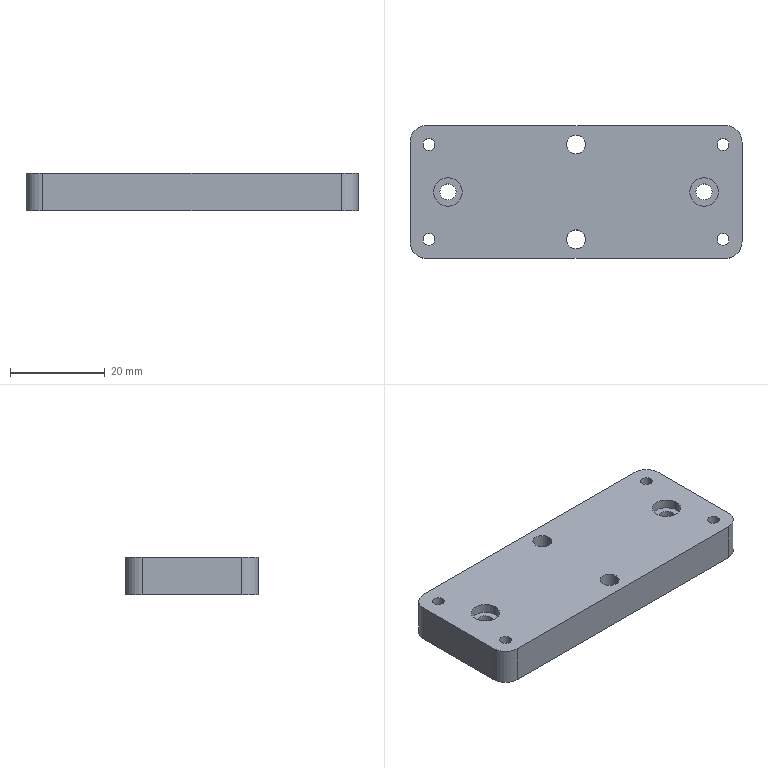Part | STEP file | 11-FG-SB01211 | 1 solid | 38 faces | box 70 x 28 x 8 mm | volume 14852 mm3 | cylinder 28 | plane 10 | commonest cylinder face diameters 2.5 x8 3.4 x4 4 x4 6 x4 6.5 x4 7 x4
STEP:
#1=CARTESIAN_POINT('',(-2.,-10.,8.));
#2=VERTEX_POINT('',#1);
#3=CARTESIAN_POINT('',(2.,-10.,8.));
#4=VERTEX_POINT('',#3);
#5=CARTESIAN_POINT('',(0.,-10.,8.));
#6=DIRECTION('',(0.,0.,1.));
#7=DIRECTION('',(1.,0.,0.));
#8=AXIS2_PLACEMENT_3D('',#5,#6,#7);
#9=CIRCLE('',#8,2.);
#10=EDGE_CURVE('',#2,#4,#9,.T.);
#11=ORIENTED_EDGE('',*,*,#10,.T.);
#12=CARTESIAN_POINT('',(2.,-10.,0.));
#13=VERTEX_POINT('',#12);
#14=CARTESIAN_POINT('',(2.,-10.,0.));
#15=DIRECTION('',(0.,0.,-1.));
#16=VECTOR('',#15,1000.);
#17=LINE('',#14,#16);
#18=EDGE_CURVE('',#4,#13,#17,.T.);
#19=ORIENTED_EDGE('',*,*,#18,.T.);
#20=CARTESIAN_POINT('',(-2.,-10.,0.));
#21=VERTEX_POINT('',#20);
#22=CARTESIAN_POINT('',(0.,-10.,0.));
#23=DIRECTION('',(0.,0.,-1.));
#24=DIRECTION('',(-1.,0.,0.));
#25=AXIS2_PLACEMENT_3D('',#22,#23,#24);
#26=CIRCLE('',#25,2.);
#27=EDGE_CURVE('',#13,#21,#26,.T.);
#28=ORIENTED_EDGE('',*,*,#27,.T.);
#29=CARTESIAN_POINT('',(-2.,-10.,0.));
#30=DIRECTION('',(0.,0.,-1.));
#31=VECTOR('',#30,1000.);
#32=LINE('',#29,#31);
#33=EDGE_CURVE('',#2,#21,#32,.T.);
#34=ORIENTED_EDGE('',*,*,#33,.F.);
#35=EDGE_LOOP('',(#11,#19,#28,#34));
#36=FACE_OUTER_BOUND('',#35,.T.);
#37=CARTESIAN_POINT('',(0.,-10.,0.));
#38=DIRECTION('',(0.,0.,-1.));
#39=DIRECTION('',(-1.,0.,0.));
#40=AXIS2_PLACEMENT_3D('',#37,#38,#39);
#41=CYLINDRICAL_SURFACE('',#40,2.);
#42=ADVANCED_FACE('',(#36),#41,.F.);
#43=CARTESIAN_POINT('',(-2.,10.,8.));
#44=VERTEX_POINT('',#43);
#45=CARTESIAN_POINT('',(2.,10.,8.));
#46=VERTEX_POINT('',#45);
#47=CARTESIAN_POINT('',(0.,10.,8.));
#48=DIRECTION('',(0.,0.,1.));
#49=DIRECTION('',(1.,0.,0.));
#50=AXIS2_PLACEMENT_3D('',#47,#48,#49);
#51=CIRCLE('',#50,2.);
#52=EDGE_CURVE('',#44,#46,#51,.T.);
#53=ORIENTED_EDGE('',*,*,#52,.T.);
#54=CARTESIAN_POINT('',(2.,10.,0.));
#55=VERTEX_POINT('',#54);
#56=CARTESIAN_POINT('',(2.,10.,0.));
#57=DIRECTION('',(0.,0.,-1.));
#58=VECTOR('',#57,1000.);
#59=LINE('',#56,#58);
#60=EDGE_CURVE('',#46,#55,#59,.T.);
#61=ORIENTED_EDGE('',*,*,#60,.T.);
#62=CARTESIAN_POINT('',(-2.,10.,0.));
#63=VERTEX_POINT('',#62);
#64=CARTESIAN_POINT('',(0.,10.,0.));
#65=DIRECTION('',(0.,0.,-1.));
#66=DIRECTION('',(-1.,0.,0.));
#67=AXIS2_PLACEMENT_3D('',#64,#65,#66);
#68=CIRCLE('',#67,2.);
#69=EDGE_CURVE('',#55,#63,#68,.T.);
#70=ORIENTED_EDGE('',*,*,#69,.T.);
#71=CARTESIAN_POINT('',(-2.,10.,0.));
#72=DIRECTION('',(0.,0.,-1.));
#73=VECTOR('',#72,1000.);
#74=LINE('',#71,#73);
#75=EDGE_CURVE('',#44,#63,#74,.T.);
#76=ORIENTED_EDGE('',*,*,#75,.F.);
#77=EDGE_LOOP('',(#53,#61,#70,#76));
#78=FACE_OUTER_BOUND('',#77,.T.);
#79=CARTESIAN_POINT('',(0.,10.,0.));
#80=DIRECTION('',(0.,0.,-1.));
#81=DIRECTION('',(-1.,0.,0.));
#82=AXIS2_PLACEMENT_3D('',#79,#80,#81);
#83=CYLINDRICAL_SURFACE('',#82,2.);
#84=ADVANCED_FACE('',(#78),#83,.F.);
#85=CARTESIAN_POINT('',(32.25,10.,8.));
#86=VERTEX_POINT('',#85);
#87=CARTESIAN_POINT('',(29.75,10.,8.));
#88=VERTEX_POINT('',#87);
#89=CARTESIAN_POINT('',(31.,10.,8.));
#90=DIRECTION('',(0.,0.,-1.));
#91=DIRECTION('',(-1.,0.,0.));
#92=AXIS2_PLACEMENT_3D('',#89,#90,#91);
#93=CIRCLE('',#92,1.25);
#94=EDGE_CURVE('',#86,#88,#93,.T.);
#95=ORIENTED_EDGE('',*,*,#94,.F.);
#96=CARTESIAN_POINT('',(32.25,10.,0.));
#97=VERTEX_POINT('',#96);
#98=CARTESIAN_POINT('',(32.25,10.,0.));
#99=DIRECTION('',(0.,0.,-1.));
#100=VECTOR('',#99,1000.);
#101=LINE('',#98,#100);
#102=EDGE_CURVE('',#86,#97,#101,.T.);
#103=ORIENTED_EDGE('',*,*,#102,.T.);
#104=CARTESIAN_POINT('',(29.75,10.,0.));
#105=VERTEX_POINT('',#104);
#106=CARTESIAN_POINT('',(31.,10.,0.));
#107=DIRECTION('',(0.,0.,-1.));
#108=DIRECTION('',(-1.,0.,0.));
#109=AXIS2_PLACEMENT_3D('',#106,#107,#108);
#110=CIRCLE('',#109,1.25);
#111=EDGE_CURVE('',#97,#105,#110,.T.);
#112=ORIENTED_EDGE('',*,*,#111,.T.);
#113=CARTESIAN_POINT('',(29.75,10.,0.));
#114=DIRECTION('',(0.,0.,-1.));
#115=VECTOR('',#114,1000.);
#116=LINE('',#113,#115);
#117=EDGE_CURVE('',#88,#105,#116,.T.);
#118=ORIENTED_EDGE('',*,*,#117,.F.);
#119=EDGE_LOOP('',(#95,#103,#112,#118));
#120=FACE_OUTER_BOUND('',#119,.T.);
#121=CARTESIAN_POINT('',(31.,10.,0.));
#122=DIRECTION('',(0.,0.,-1.));
#123=DIRECTION('',(-1.,0.,0.));
#124=AXIS2_PLACEMENT_3D('',#121,#122,#123);
#125=CYLINDRICAL_SURFACE('',#124,1.25);
#126=ADVANCED_FACE('',(#120),#125,.F.);
#127=CARTESIAN_POINT('',(32.25,-10.,8.));
#128=VERTEX_POINT('',#127);
#129=CARTESIAN_POINT('',(29.75,-10.,8.));
#130=VERTEX_POINT('',#129);
#131=CARTESIAN_POINT('',(31.,-10.,8.));
#132=DIRECTION('',(0.,0.,-1.));
#133=DIRECTION('',(-1.,0.,0.));
#134=AXIS2_PLACEMENT_3D('',#131,#132,#133);
#135=CIRCLE('',#134,1.25);
#136=EDGE_CURVE('',#128,#130,#135,.T.);
#137=ORIENTED_EDGE('',*,*,#136,.F.);
#138=CARTESIAN_POINT('',(32.25,-10.,0.));
#139=VERTEX_POINT('',#138);
#140=CARTESIAN_POINT('',(32.25,-10.,0.));
#141=DIRECTION('',(0.,0.,-1.));
#142=VECTOR('',#141,1000.);
#143=LINE('',#140,#142);
#144=EDGE_CURVE('',#128,#139,#143,.T.);
#145=ORIENTED_EDGE('',*,*,#144,.T.);
#146=CARTESIAN_POINT('',(29.75,-10.,0.));
#147=VERTEX_POINT('',#146);
#148=CARTESIAN_POINT('',(31.,-10.,0.));
#149=DIRECTION('',(0.,0.,-1.));
#150=DIRECTION('',(-1.,0.,0.));
#151=AXIS2_PLACEMENT_3D('',#148,#149,#150);
#152=CIRCLE('',#151,1.25);
#153=EDGE_CURVE('',#139,#147,#152,.T.);
#154=ORIENTED_EDGE('',*,*,#153,.T.);
#155=CARTESIAN_POINT('',(29.75,-10.,0.));
#156=DIRECTION('',(0.,0.,-1.));
#157=VECTOR('',#156,1000.);
#158=LINE('',#155,#157);
#159=EDGE_CURVE('',#130,#147,#158,.T.);
#160=ORIENTED_EDGE('',*,*,#159,.F.);
#161=EDGE_LOOP('',(#137,#145,#154,#160));
#162=FACE_OUTER_BOUND('',#161,.T.);
#163=CARTESIAN_POINT('',(31.,-10.,0.));
#164=DIRECTION('',(0.,0.,-1.));
#165=DIRECTION('',(-1.,0.,0.));
#166=AXIS2_PLACEMENT_3D('',#163,#164,#165);
#167=CYLINDRICAL_SURFACE('',#166,1.25);
#168=ADVANCED_FACE('',(#162),#167,.F.);
#169=CARTESIAN_POINT('',(-29.75,-10.,8.));
#170=VERTEX_POINT('',#169);
#171=CARTESIAN_POINT('',(-32.25,-10.,8.));
#172=VERTEX_POINT('',#171);
#173=CARTESIAN_POINT('',(-31.,-10.,8.));
#174=DIRECTION('',(0.,0.,-1.));
#175=DIRECTION('',(-1.,0.,0.));
#176=AXIS2_PLACEMENT_3D('',#173,#174,#175);
#177=CIRCLE('',#176,1.25);
#178=EDGE_CURVE('',#170,#172,#177,.T.);
#179=ORIENTED_EDGE('',*,*,#178,.F.);
#180=CARTESIAN_POINT('',(-29.75,-10.,0.));
#181=VERTEX_POINT('',#180);
#182=CARTESIAN_POINT('',(-29.75,-10.,0.));
#183=DIRECTION('',(0.,0.,-1.));
#184=VECTOR('',#183,1000.);
#185=LINE('',#182,#184);
#186=EDGE_CURVE('',#170,#181,#185,.T.);
#187=ORIENTED_EDGE('',*,*,#186,.T.);
#188=CARTESIAN_POINT('',(-32.25,-10.,0.));
#189=VERTEX_POINT('',#188);
#190=CARTESIAN_POINT('',(-31.,-10.,0.));
#191=DIRECTION('',(0.,0.,-1.));
#192=DIRECTION('',(-1.,0.,0.));
#193=AXIS2_PLACEMENT_3D('',#190,#191,#192);
#194=CIRCLE('',#193,1.25);
#195=EDGE_CURVE('',#181,#189,#194,.T.);
#196=ORIENTED_EDGE('',*,*,#195,.T.);
#197=CARTESIAN_POINT('',(-32.25,-10.,0.));
#198=DIRECTION('',(0.,0.,-1.));
#199=VECTOR('',#198,1000.);
#200=LINE('',#197,#199);
#201=EDGE_CURVE('',#172,#189,#200,.T.);
#202=ORIENTED_EDGE('',*,*,#201,.F.);
#203=EDGE_LOOP('',(#179,#187,#196,#202));
#204=FACE_OUTER_BOUND('',#203,.T.);
#205=CARTESIAN_POINT('',(-31.,-10.,0.));
#206=DIRECTION('',(0.,0.,-1.));
#207=DIRECTION('',(-1.,0.,0.));
#208=AXIS2_PLACEMENT_3D('',#205,#206,#207);
#209=CYLINDRICAL_SURFACE('',#208,1.25);
#210=ADVANCED_FACE('',(#204),#209,.F.);
#211=CARTESIAN_POINT('',(-29.75,10.,8.));
#212=VERTEX_POINT('',#211);
#213=CARTESIAN_POINT('',(-32.25,10.,8.));
#214=VERTEX_POINT('',#213);
#215=CARTESIAN_POINT('',(-31.,10.,8.));
#216=DIRECTION('',(0.,0.,-1.));
#217=DIRECTION('',(-1.,0.,0.));
#218=AXIS2_PLACEMENT_3D('',#215,#216,#217);
#219=CIRCLE('',#218,1.25);
#220=EDGE_CURVE('',#212,#214,#219,.T.);
#221=ORIENTED_EDGE('',*,*,#220,.F.);
#222=CARTESIAN_POINT('',(-29.75,10.,0.));
#223=VERTEX_POINT('',#222);
#224=CARTESIAN_POINT('',(-29.75,10.,0.));
#225=DIRECTION('',(0.,0.,-1.));
#226=VECTOR('',#225,1000.);
#227=LINE('',#224,#226);
#228=EDGE_CURVE('',#212,#223,#227,.T.);
#229=ORIENTED_EDGE('',*,*,#228,.T.);
#230=CARTESIAN_POINT('',(-32.25,10.,0.));
#231=VERTEX_POINT('',#230);
#232=CARTESIAN_POINT('',(-31.,10.,0.));
#233=DIRECTION('',(0.,0.,-1.));
#234=DIRECTION('',(-1.,0.,0.));
#235=AXIS2_PLACEMENT_3D('',#232,#233,#234);
#236=CIRCLE('',#235,1.25);
#237=EDGE_CURVE('',#223,#231,#236,.T.);
#238=ORIENTED_EDGE('',*,*,#237,.T.);
#239=CARTESIAN_POINT('',(-32.25,10.,0.));
#240=DIRECTION('',(0.,0.,-1.));
#241=VECTOR('',#240,1000.);
#242=LINE('',#239,#241);
#243=EDGE_CURVE('',#214,#231,#242,.T.);
#244=ORIENTED_EDGE('',*,*,#243,.F.);
#245=EDGE_LOOP('',(#221,#229,#238,#244));
#246=FACE_OUTER_BOUND('',#245,.T.);
#247=CARTESIAN_POINT('',(-31.,10.,0.));
#248=DIRECTION('',(0.,0.,-1.));
#249=DIRECTION('',(-1.,0.,0.));
#250=AXIS2_PLACEMENT_3D('',#247,#248,#249);
#251=CYLINDRICAL_SURFACE('',#250,1.25);
#252=ADVANCED_FACE('',(#246),#251,.F.);
#253=CARTESIAN_POINT('',(-23.75,0.,3.4));
#254=VERTEX_POINT('',#253);
#255=CARTESIAN_POINT('',(-30.25,0.,3.4));
#256=VERTEX_POINT('',#255);
#257=CARTESIAN_POINT('',(-27.,0.,3.4));
#258=DIRECTION('',(0.,0.,-1.));
#259=DIRECTION('',(-1.,0.,0.));
#260=AXIS2_PLACEMENT_3D('',#257,#258,#259);
#261=CIRCLE('',#260,3.25);
#262=EDGE_CURVE('',#254,#256,#261,.T.);
#263=ORIENTED_EDGE('',*,*,#262,.F.);
#264=CARTESIAN_POINT('',(-23.75,0.,0.));
#265=VERTEX_POINT('',#264);
#266=CARTESIAN_POINT('',(-23.75,0.,0.));
#267=DIRECTION('',(0.,0.,-1.));
#268=VECTOR('',#267,1000.);
#269=LINE('',#266,#268);
#270=EDGE_CURVE('',#254,#265,#269,.T.);
#271=ORIENTED_EDGE('',*,*,#270,.T.);
#272=CARTESIAN_POINT('',(-30.25,0.,0.));
#273=VERTEX_POINT('',#272);
#274=CARTESIAN_POINT('',(-27.,0.,0.));
#275=DIRECTION('',(0.,0.,-1.));
#276=DIRECTION('',(-1.,0.,0.));
#277=AXIS2_PLACEMENT_3D('',#274,#275,#276);
#278=CIRCLE('',#277,3.25);
#279=EDGE_CURVE('',#265,#273,#278,.T.);
#280=ORIENTED_EDGE('',*,*,#279,.T.);
#281=CARTESIAN_POINT('',(-30.25,0.,0.));
#282=DIRECTION('',(0.,0.,-1.));
#283=VECTOR('',#282,1000.);
#284=LINE('',#281,#283);
#285=EDGE_CURVE('',#256,#273,#284,.T.);
#286=ORIENTED_EDGE('',*,*,#285,.F.);
#287=EDGE_LOOP('',(#263,#271,#280,#286));
#288=FACE_OUTER_BOUND('',#287,.T.);
#289=CARTESIAN_POINT('',(-27.,0.,0.));
#290=DIRECTION('',(0.,0.,-1.));
#291=DIRECTION('',(-1.,0.,0.));
#292=AXIS2_PLACEMENT_3D('',#289,#290,#291);
#293=CYLINDRICAL_SURFACE('',#292,3.25);
#294=ADVANCED_FACE('',(#288),#293,.F.);
#295=CARTESIAN_POINT('',(-25.3,0.,6.));
#296=VERTEX_POINT('',#295);
#297=CARTESIAN_POINT('',(-28.7,0.,6.));
#298=VERTEX_POINT('',#297);
#299=CARTESIAN_POINT('',(-27.,0.,6.));
#300=DIRECTION('',(0.,0.,-1.));
#301=DIRECTION('',(-1.,0.,0.));
#302=AXIS2_PLACEMENT_3D('',#299,#300,#301);
#303=CIRCLE('',#302,1.7);
#304=EDGE_CURVE('',#296,#298,#303,.T.);
#305=ORIENTED_EDGE('',*,*,#304,.F.);
#306=CARTESIAN_POINT('',(-25.3,0.,3.4));
#307=VERTEX_POINT('',#306);
#308=CARTESIAN_POINT('',(-25.3,0.,0.));
#309=DIRECTION('',(0.,0.,-1.));
#310=VECTOR('',#309,1000.);
#311=LINE('',#308,#310);
#312=EDGE_CURVE('',#296,#307,#311,.T.);
#313=ORIENTED_EDGE('',*,*,#312,.T.);
#314=CARTESIAN_POINT('',(-28.7,0.,3.4));
#315=VERTEX_POINT('',#314);
#316=CARTESIAN_POINT('',(-27.,0.,3.4));
#317=DIRECTION('',(0.,0.,-1.));
#318=DIRECTION('',(-1.,0.,0.));
#319=AXIS2_PLACEMENT_3D('',#316,#317,#318);
#320=CIRCLE('',#319,1.7);
#321=EDGE_CURVE('',#307,#315,#320,.T.);
#322=ORIENTED_EDGE('',*,*,#321,.T.);
#323=CARTESIAN_POINT('',(-28.7,0.,0.));
#324=DIRECTION('',(0.,0.,-1.));
#325=VECTOR('',#324,1000.);
#326=LINE('',#323,#325);
#327=EDGE_CURVE('',#298,#315,#326,.T.);
#328=ORIENTED_EDGE('',*,*,#327,.F.);
#329=EDGE_LOOP('',(#305,#313,#322,#328));
#330=FACE_OUTER_BOUND('',#329,.T.);
#331=CARTESIAN_POINT('',(-27.,0.,0.));
#332=DIRECTION('',(0.,0.,-1.));
#333=DIRECTION('',(-1.,0.,0.));
#334=AXIS2_PLACEMENT_3D('',#331,#332,#333);
#335=CYLINDRICAL_SURFACE('',#334,1.7);
#336=ADVANCED_FACE('',(#330),#335,.F.);
#337=CARTESIAN_POINT('',(30.25,0.,3.4));
#338=VERTEX_POINT('',#337);
#339=CARTESIAN_POINT('',(23.75,0.,3.4));
#340=VERTEX_POINT('',#339);
#341=CARTESIAN_POINT('',(27.,0.,3.4));
#342=DIRECTION('',(0.,0.,-1.));
#343=DIRECTION('',(-1.,0.,0.));
#344=AXIS2_PLACEMENT_3D('',#341,#342,#343);
#345=CIRCLE('',#344,3.25);
#346=EDGE_CURVE('',#338,#340,#345,.T.);
#347=ORIENTED_EDGE('',*,*,#346,.F.);
#348=CARTESIAN_POINT('',(30.25,0.,0.));
#349=VERTEX_POINT('',#348);
#350=CARTESIAN_POINT('',(30.25,0.,0.));
#351=DIRECTION('',(0.,0.,-1.));
#352=VECTOR('',#351,1000.);
#353=LINE('',#350,#352);
#354=EDGE_CURVE('',#338,#349,#353,.T.);
#355=ORIENTED_EDGE('',*,*,#354,.T.);
#356=CARTESIAN_POINT('',(23.75,0.,0.));
#357=VERTEX_POINT('',#356);
#358=CARTESIAN_POINT('',(27.,0.,0.));
#359=DIRECTION('',(0.,0.,-1.));
#360=DIRECTION('',(-1.,0.,0.));
#361=AXIS2_PLACEMENT_3D('',#358,#359,#360);
#362=CIRCLE('',#361,3.25);
#363=EDGE_CURVE('',#349,#357,#362,.T.);
#364=ORIENTED_EDGE('',*,*,#363,.T.);
#365=CARTESIAN_POINT('',(23.75,0.,0.));
#366=DIRECTION('',(0.,0.,-1.));
#367=VECTOR('',#366,1000.);
#368=LINE('',#365,#367);
#369=EDGE_CURVE('',#340,#357,#368,.T.);
#370=ORIENTED_EDGE('',*,*,#369,.F.);
#371=EDGE_LOOP('',(#347,#355,#364,#370));
#372=FACE_OUTER_BOUND('',#371,.T.);
#373=CARTESIAN_POINT('',(27.,0.,0.));
#374=DIRECTION('',(0.,0.,-1.));
#375=DIRECTION('',(-1.,0.,0.));
#376=AXIS2_PLACEMENT_3D('',#373,#374,#375);
#377=CYLINDRICAL_SURFACE('',#376,3.25);
#378=ADVANCED_FACE('',(#372),#377,.F.);
#379=CARTESIAN_POINT('',(25.3,0.,6.));
#380=VERTEX_POINT('',#379);
#381=CARTESIAN_POINT('',(28.7,0.,6.));
#382=VERTEX_POINT('',#381);
#383=CARTESIAN_POINT('',(27.,0.,6.));
#384=DIRECTION('',(0.,0.,1.));
#385=DIRECTION('',(1.,0.,0.));
#386=AXIS2_PLACEMENT_3D('',#383,#384,#385);
#387=CIRCLE('',#386,1.7);
#388=EDGE_CURVE('',#380,#382,#387,.T.);
#389=ORIENTED_EDGE('',*,*,#388,.T.);
#390=CARTESIAN_POINT('',(28.7,0.,3.4));
#391=VERTEX_POINT('',#390);
#392=CARTESIAN_POINT('',(28.7,0.,0.));
#393=DIRECTION('',(0.,0.,-1.));
#394=VECTOR('',#393,1000.);
#395=LINE('',#392,#394);
#396=EDGE_CURVE('',#382,#391,#395,.T.);
#397=ORIENTED_EDGE('',*,*,#396,.T.);
#398=CARTESIAN_POINT('',(25.3,0.,3.4));
#399=VERTEX_POINT('',#398);
#400=CARTESIAN_POINT('',(27.,0.,3.4));
#401=DIRECTION('',(0.,0.,-1.));
#402=DIRECTION('',(-1.,0.,0.));
#403=AXIS2_PLACEMENT_3D('',#400,#401,#402);
#404=CIRCLE('',#403,1.7);
#405=EDGE_CURVE('',#391,#399,#404,.T.);
#406=ORIENTED_EDGE('',*,*,#405,.T.);
#407=CARTESIAN_POINT('',(25.3,0.,0.));
#408=DIRECTION('',(0.,0.,-1.));
#409=VECTOR('',#408,1000.);
#410=LINE('',#407,#409);
#411=EDGE_CURVE('',#380,#399,#410,.T.);
#412=ORIENTED_EDGE('',*,*,#411,.F.);
#413=EDGE_LOOP('',(#389,#397,#406,#412));
#414=FACE_OUTER_BOUND('',#413,.T.);
#415=CARTESIAN_POINT('',(27.,0.,0.));
#416=DIRECTION('',(0.,0.,-1.));
#417=DIRECTION('',(-1.,0.,0.));
#418=AXIS2_PLACEMENT_3D('',#415,#416,#417);
#419=CYLINDRICAL_SURFACE('',#418,1.7);
#420=ADVANCED_FACE('',(#414),#419,.F.);
#421=CARTESIAN_POINT('',(-30.,0.,6.));
#422=VERTEX_POINT('',#421);
#423=CARTESIAN_POINT('',(-24.,0.,6.));
#424=VERTEX_POINT('',#423);
#425=CARTESIAN_POINT('',(-27.,0.,6.));
#426=DIRECTION('',(0.,0.,1.));
#427=DIRECTION('',(-1.,0.,0.));
#428=AXIS2_PLACEMENT_3D('',#425,#426,#427);
#429=CIRCLE('',#428,3.);
#430=EDGE_CURVE('',#422,#424,#429,.T.);
#431=ORIENTED_EDGE('',*,*,#430,.F.);
#432=CARTESIAN_POINT('',(-30.,0.,8.));
#433=VERTEX_POINT('',#432);
#434=CARTESIAN_POINT('',(-30.,0.,6.));
#435=DIRECTION('',(0.,0.,1.));
#436=VECTOR('',#435,1000.);
#437=LINE('',#434,#436);
#438=EDGE_CURVE('',#422,#433,#437,.T.);
#439=ORIENTED_EDGE('',*,*,#438,.T.);
#440=CARTESIAN_POINT('',(-24.,0.,8.));
#441=VERTEX_POINT('',#440);
#442=CARTESIAN_POINT('',(-27.,0.,8.));
#443=DIRECTION('',(0.,0.,1.));
#444=DIRECTION('',(-1.,0.,0.));
#445=AXIS2_PLACEMENT_3D('',#442,#443,#444);
#446=CIRCLE('',#445,3.);
#447=EDGE_CURVE('',#433,#441,#446,.T.);
#448=ORIENTED_EDGE('',*,*,#447,.T.);
#449=CARTESIAN_POINT('',(-24.,0.,6.));
#450=DIRECTION('',(0.,0.,1.));
#451=VECTOR('',#450,1000.);
#452=LINE('',#449,#451);
#453=EDGE_CURVE('',#424,#441,#452,.T.);
#454=ORIENTED_EDGE('',*,*,#453,.F.);
#455=EDGE_LOOP('',(#431,#439,#448,#454));
#456=FACE_OUTER_BOUND('',#455,.T.);
#457=CARTESIAN_POINT('',(-27.,0.,6.));
#458=DIRECTION('',(0.,0.,1.));
#459=DIRECTION('',(1.,0.,0.));
#460=AXIS2_PLACEMENT_3D('',#457,#458,#459);
#461=CYLINDRICAL_SURFACE('',#460,3.);
#462=ADVANCED_FACE('',(#456),#461,.F.);
#463=CARTESIAN_POINT('',(24.,0.,6.));
#464=VERTEX_POINT('',#463);
#465=CARTESIAN_POINT('',(30.,0.,6.));
#466=VERTEX_POINT('',#465);
#467=CARTESIAN_POINT('',(27.,0.,6.));
#468=DIRECTION('',(0.,0.,1.));
#469=DIRECTION('',(1.,0.,0.));
#470=AXIS2_PLACEMENT_3D('',#467,#468,#469);
#471=CIRCLE('',#470,3.);
#472=EDGE_CURVE('',#464,#466,#471,.T.);
#473=ORIENTED_EDGE('',*,*,#472,.F.);
#474=CARTESIAN_POINT('',(24.,0.,8.));
#475=VERTEX_POINT('',#474);
#476=CARTESIAN_POINT('',(24.,0.,6.));
#477=DIRECTION('',(0.,0.,1.));
#478=VECTOR('',#477,1000.);
#479=LINE('',#476,#478);
#480=EDGE_CURVE('',#464,#475,#479,.T.);
#481=ORIENTED_EDGE('',*,*,#480,.T.);
#482=CARTESIAN_POINT('',(30.,0.,8.));
#483=VERTEX_POINT('',#482);
#484=CARTESIAN_POINT('',(27.,0.,8.));
#485=DIRECTION('',(0.,0.,1.));
#486=DIRECTION('',(1.,0.,0.));
#487=AXIS2_PLACEMENT_3D('',#484,#485,#486);
#488=CIRCLE('',#487,3.);
#489=EDGE_CURVE('',#475,#483,#488,.T.);
#490=ORIENTED_EDGE('',*,*,#489,.T.);
#491=CARTESIAN_POINT('',(30.,0.,6.));
#492=DIRECTION('',(0.,0.,1.));
#493=VECTOR('',#492,1000.);
#494=LINE('',#491,#493);
#495=EDGE_CURVE('',#466,#483,#494,.T.);
#496=ORIENTED_EDGE('',*,*,#495,.F.);
#497=EDGE_LOOP('',(#473,#481,#490,#496));
#498=FACE_OUTER_BOUND('',#497,.T.);
#499=CARTESIAN_POINT('',(27.,0.,6.));
#500=DIRECTION('',(0.,0.,1.));
#501=DIRECTION('',(1.,0.,0.));
#502=AXIS2_PLACEMENT_3D('',#499,#500,#501);
#503=CYLINDRICAL_SURFACE('',#502,3.);
#504=ADVANCED_FACE('',(#498),#503,.F.);
#505=CARTESIAN_POINT('',(35.,-10.5,0.));
#506=VERTEX_POINT('',#505);
#507=CARTESIAN_POINT('',(35.,10.5,0.));
#508=VERTEX_POINT('',#507);
#509=CARTESIAN_POINT('',(35.,14.,0.));
#510=DIRECTION('',(0.,1.,0.));
#511=VECTOR('',#510,1000.);
#512=LINE('',#509,#511);
#513=EDGE_CURVE('',#506,#508,#512,.T.);
#514=ORIENTED_EDGE('',*,*,#513,.T.);
#515=CARTESIAN_POINT('',(35.,10.5,8.));
#516=VERTEX_POINT('',#515);
#517=CARTESIAN_POINT('',(35.,10.5,8.));
#518=DIRECTION('',(0.,0.,1.));
#519=VECTOR('',#518,1000.);
#520=LINE('',#517,#519);
#521=EDGE_CURVE('',#508,#516,#520,.T.);
#522=ORIENTED_EDGE('',*,*,#521,.T.);
#523=CARTESIAN_POINT('',(35.,-10.5,8.));
#524=VERTEX_POINT('',#523);
#525=CARTESIAN_POINT('',(35.,14.,8.));
#526=DIRECTION('',(0.,1.,0.));
#527=VECTOR('',#526,1000.);
#528=LINE('',#525,#527);
#529=EDGE_CURVE('',#524,#516,#528,.T.);
#530=ORIENTED_EDGE('',*,*,#529,.F.);
#531=CARTESIAN_POINT('',(35.,-10.5,8.));
#532=DIRECTION('',(0.,0.,-1.));
#533=VECTOR('',#532,1000.);
#534=LINE('',#531,#533);
#535=EDGE_CURVE('',#524,#506,#534,.T.);
#536=ORIENTED_EDGE('',*,*,#535,.T.);
#537=EDGE_LOOP('',(#514,#522,#530,#536));
#538=FACE_OUTER_BOUND('',#537,.T.);
#539=CARTESIAN_POINT('',(35.,14.,8.));
#540=DIRECTION('',(-1.,0.,0.));
#541=DIRECTION('',(0.,0.,1.));
#542=AXIS2_PLACEMENT_3D('',#539,#540,#541);
#543=PLANE('',#542);
#544=ADVANCED_FACE('',(#538),#543,.F.);
#545=CARTESIAN_POINT('',(31.5,14.,8.));
#546=VERTEX_POINT('',#545);
#547=CARTESIAN_POINT('',(-31.5,14.,8.));
#548=VERTEX_POINT('',#547);
#549=CARTESIAN_POINT('',(-35.,14.,8.));
#550=DIRECTION('',(-1.,0.,0.));
#551=VECTOR('',#550,1000.);
#552=LINE('',#549,#551);
#553=EDGE_CURVE('',#546,#548,#552,.T.);
#554=ORIENTED_EDGE('',*,*,#553,.F.);
#555=CARTESIAN_POINT('',(31.5,14.,0.));
#556=VERTEX_POINT('',#555);
#557=CARTESIAN_POINT('',(31.5,14.,8.));
#558=DIRECTION('',(0.,0.,-1.));
#559=VECTOR('',#558,1000.);
#560=LINE('',#557,#559);
#561=EDGE_CURVE('',#546,#556,#560,.T.);
#562=ORIENTED_EDGE('',*,*,#561,.T.);
#563=CARTESIAN_POINT('',(-31.5,14.,0.));
#564=VERTEX_POINT('',#563);
#565=CARTESIAN_POINT('',(-35.,14.,0.));
#566=DIRECTION('',(-1.,0.,0.));
#567=VECTOR('',#566,1000.);
#568=LINE('',#565,#567);
#569=EDGE_CURVE('',#556,#564,#568,.T.);
#570=ORIENTED_EDGE('',*,*,#569,.T.);
#571=CARTESIAN_POINT('',(-31.5,14.,8.));
#572=DIRECTION('',(0.,0.,1.));
#573=VECTOR('',#572,1000.);
#574=LINE('',#571,#573);
#575=EDGE_CURVE('',#564,#548,#574,.T.);
#576=ORIENTED_EDGE('',*,*,#575,.T.);
#577=EDGE_LOOP('',(#554,#562,#570,#576));
#578=FACE_OUTER_BOUND('',#577,.T.);
#579=CARTESIAN_POINT('',(-35.,14.,8.));
#580=DIRECTION('',(0.,-1.,0.));
#581=DIRECTION('',(0.,0.,-1.));
#582=AXIS2_PLACEMENT_3D('',#579,#580,#581);
#583=PLANE('',#582);
#584=ADVANCED_FACE('',(#578),#583,.F.);
#585=CARTESIAN_POINT('',(-35.,10.5,0.));
#586=VERTEX_POINT('',#585);
#587=CARTESIAN_POINT('',(-35.,-10.5,0.));
#588=VERTEX_POINT('',#587);
#589=CARTESIAN_POINT('',(-35.,14.,0.));
#590=DIRECTION('',(0.,-1.,0.));
#591=VECTOR('',#590,1000.);
#592=LINE('',#589,#591);
#593=EDGE_CURVE('',#586,#588,#592,.T.);
#594=ORIENTED_EDGE('',*,*,#593,.T.);
#595=CARTESIAN_POINT('',(-35.,-10.5,8.));
#596=VERTEX_POINT('',#595);
#597=CARTESIAN_POINT('',(-35.,-10.5,8.));
#598=DIRECTION('',(0.,0.,1.));
#599=VECTOR('',#598,1000.);
#600=LINE('',#597,#599);
#601=EDGE_CURVE('',#588,#596,#600,.T.);
#602=ORIENTED_EDGE('',*,*,#601,.T.);
#603=CARTESIAN_POINT('',(-35.,10.5,8.));
#604=VERTEX_POINT('',#603);
#605=CARTESIAN_POINT('',(-35.,14.,8.));
#606=DIRECTION('',(0.,-1.,0.));
#607=VECTOR('',#606,1000.);
#608=LINE('',#605,#607);
#609=EDGE_CURVE('',#604,#596,#608,.T.);
#610=ORIENTED_EDGE('',*,*,#609,.F.);
#611=CARTESIAN_POINT('',(-35.,10.5,8.));
#612=DIRECTION('',(0.,0.,-1.));
#613=VECTOR('',#612,1000.);
#614=LINE('',#611,#613);
#615=EDGE_CURVE('',#604,#586,#614,.T.);
#616=ORIENTED_EDGE('',*,*,#615,.T.);
#617=EDGE_LOOP('',(#594,#602,#610,#616));
#618=FACE_OUTER_BOUND('',#617,.T.);
#619=CARTESIAN_POINT('',(-35.,14.,8.));
#620=DIRECTION('',(1.,0.,0.));
#621=DIRECTION('',(0.,1.,0.));
#622=AXIS2_PLACEMENT_3D('',#619,#620,#621);
#623=PLANE('',#622);
#624=ADVANCED_FACE('',(#618),#623,.F.);
#625=CARTESIAN_POINT('',(-31.5,-14.,0.));
#626=VERTEX_POINT('',#625);
#627=CARTESIAN_POINT('',(31.5,-14.,0.));
#628=VERTEX_POINT('',#627);
#629=CARTESIAN_POINT('',(-35.,-14.,0.));
#630=DIRECTION('',(1.,0.,0.));
#631=VECTOR('',#630,1000.);
#632=LINE('',#629,#631);
#633=EDGE_CURVE('',#626,#628,#632,.T.);
#634=ORIENTED_EDGE('',*,*,#633,.T.);
#635=CARTESIAN_POINT('',(31.5,-14.,8.));
#636=VERTEX_POINT('',#635);
#637=CARTESIAN_POINT('',(31.5,-14.,8.));
#638=DIRECTION('',(0.,0.,1.));
#639=VECTOR('',#638,1000.);
#640=LINE('',#637,#639);
#641=EDGE_CURVE('',#628,#636,#640,.T.);
#642=ORIENTED_EDGE('',*,*,#641,.T.);
#643=CARTESIAN_POINT('',(-31.5,-14.,8.));
#644=VERTEX_POINT('',#643);
#645=CARTESIAN_POINT('',(-35.,-14.,8.));
#646=DIRECTION('',(1.,0.,0.));
#647=VECTOR('',#646,1000.);
#648=LINE('',#645,#647);
#649=EDGE_CURVE('',#644,#636,#648,.T.);
#650=ORIENTED_EDGE('',*,*,#649,.F.);
#651=CARTESIAN_POINT('',(-31.5,-14.,8.));
#652=DIRECTION('',(0.,0.,-1.));
#653=VECTOR('',#652,1000.);
#654=LINE('',#651,#653);
#655=EDGE_CURVE('',#644,#626,#654,.T.);
#656=ORIENTED_EDGE('',*,*,#655,.T.);
#657=EDGE_LOOP('',(#634,#642,#650,#656));
#658=FACE_OUTER_BOUND('',#657,.T.);
#659=CARTESIAN_POINT('',(-35.,-14.,8.));
#660=DIRECTION('',(0.,1.,0.));
#661=DIRECTION('',(0.,0.,1.));
#662=AXIS2_PLACEMENT_3D('',#659,#660,#661);
#663=PLANE('',#662);
#664=ADVANCED_FACE('',(#658),#663,.F.);
#665=ORIENTED_EDGE('',*,*,#10,.F.);
#666=CARTESIAN_POINT('',(0.,-10.,8.));
#667=DIRECTION('',(0.,0.,1.));
#668=DIRECTION('',(1.,0.,0.));
#669=AXIS2_PLACEMENT_3D('',#666,#667,#668);
#670=CIRCLE('',#669,2.);
#671=EDGE_CURVE('',#4,#2,#670,.T.);
#672=ORIENTED_EDGE('',*,*,#671,.F.);
#673=EDGE_LOOP('',(#665,#672));
#674=FACE_BOUND('',#673,.T.);
#675=ORIENTED_EDGE('',*,*,#52,.F.);
#676=CARTESIAN_POINT('',(0.,10.,8.));
#677=DIRECTION('',(0.,0.,1.));
#678=DIRECTION('',(1.,0.,0.));
#679=AXIS2_PLACEMENT_3D('',#676,#677,#678);
#680=CIRCLE('',#679,2.);
#681=EDGE_CURVE('',#46,#44,#680,.T.);
#682=ORIENTED_EDGE('',*,*,#681,.F.);
#683=EDGE_LOOP('',(#675,#682));
#684=FACE_BOUND('',#683,.T.);
#685=CARTESIAN_POINT('',(31.,10.,8.));
#686=DIRECTION('',(0.,0.,-1.));
#687=DIRECTION('',(-1.,0.,0.));
#688=AXIS2_PLACEMENT_3D('',#685,#686,#687);
#689=CIRCLE('',#688,1.25);
#690=EDGE_CURVE('',#88,#86,#689,.T.);
#691=ORIENTED_EDGE('',*,*,#690,.T.);
#692=ORIENTED_EDGE('',*,*,#94,.T.);
#693=EDGE_LOOP('',(#691,#692));
#694=FACE_BOUND('',#693,.T.);
#695=CARTESIAN_POINT('',(31.,-10.,8.));
#696=DIRECTION('',(0.,0.,-1.));
#697=DIRECTION('',(-1.,0.,0.));
#698=AXIS2_PLACEMENT_3D('',#695,#696,#697);
#699=CIRCLE('',#698,1.25);
#700=EDGE_CURVE('',#130,#128,#699,.T.);
#701=ORIENTED_EDGE('',*,*,#700,.T.);
#702=ORIENTED_EDGE('',*,*,#136,.T.);
#703=EDGE_LOOP('',(#701,#702));
#704=FACE_BOUND('',#703,.T.);
#705=CARTESIAN_POINT('',(-31.,-10.,8.));
#706=DIRECTION('',(0.,0.,-1.));
#707=DIRECTION('',(-1.,0.,0.));
#708=AXIS2_PLACEMENT_3D('',#705,#706,#707);
#709=CIRCLE('',#708,1.25);
#710=EDGE_CURVE('',#172,#170,#709,.T.);
#711=ORIENTED_EDGE('',*,*,#710,.T.);
#712=ORIENTED_EDGE('',*,*,#178,.T.);
#713=EDGE_LOOP('',(#711,#712));
#714=FACE_BOUND('',#713,.T.);
#715=CARTESIAN_POINT('',(-31.,10.,8.));
#716=DIRECTION('',(0.,0.,-1.));
#717=DIRECTION('',(-1.,0.,0.));
#718=AXIS2_PLACEMENT_3D('',#715,#716,#717);
#719=CIRCLE('',#718,1.25);
#720=EDGE_CURVE('',#214,#212,#719,.T.);
#721=ORIENTED_EDGE('',*,*,#720,.T.);
#722=ORIENTED_EDGE('',*,*,#220,.T.);
#723=EDGE_LOOP('',(#721,#722));
#724=FACE_BOUND('',#723,.T.);
#725=CARTESIAN_POINT('',(-27.,0.,8.));
#726=DIRECTION('',(0.,0.,1.));
#727=DIRECTION('',(-1.,0.,0.));
#728=AXIS2_PLACEMENT_3D('',#725,#726,#727);
#729=CIRCLE('',#728,3.);
#730=EDGE_CURVE('',#441,#433,#729,.T.);
#731=ORIENTED_EDGE('',*,*,#730,.F.);
#732=ORIENTED_EDGE('',*,*,#447,.F.);
#733=EDGE_LOOP('',(#731,#732));
#734=FACE_BOUND('',#733,.T.);
#735=CARTESIAN_POINT('',(27.,0.,8.));
#736=DIRECTION('',(0.,0.,1.));
#737=DIRECTION('',(1.,0.,0.));
#738=AXIS2_PLACEMENT_3D('',#735,#736,#737);
#739=CIRCLE('',#738,3.);
#740=EDGE_CURVE('',#483,#475,#739,.T.);
#741=ORIENTED_EDGE('',*,*,#740,.F.);
#742=ORIENTED_EDGE('',*,*,#489,.F.);
#743=EDGE_LOOP('',(#741,#742));
#744=FACE_BOUND('',#743,.T.);
#745=ORIENTED_EDGE('',*,*,#529,.T.);
#746=CARTESIAN_POINT('',(31.5,10.5,8.));
#747=DIRECTION('',(0.,0.,1.));
#748=DIRECTION('',(1.,0.,0.));
#749=AXIS2_PLACEMENT_3D('',#746,#747,#748);
#750=CIRCLE('',#749,3.5);
#751=EDGE_CURVE('',#516,#546,#750,.T.);
#752=ORIENTED_EDGE('',*,*,#751,.T.);
#753=ORIENTED_EDGE('',*,*,#553,.T.);
#754=CARTESIAN_POINT('',(-31.5,10.5,8.));
#755=DIRECTION('',(0.,0.,1.));
#756=DIRECTION('',(1.,0.,0.));
#757=AXIS2_PLACEMENT_3D('',#754,#755,#756);
#758=CIRCLE('',#757,3.5);
#759=EDGE_CURVE('',#548,#604,#758,.T.);
#760=ORIENTED_EDGE('',*,*,#759,.T.);
#761=ORIENTED_EDGE('',*,*,#609,.T.);
#762=CARTESIAN_POINT('',(-31.5,-10.5,8.));
#763=DIRECTION('',(0.,0.,1.));
#764=DIRECTION('',(1.,0.,0.));
#765=AXIS2_PLACEMENT_3D('',#762,#763,#764);
#766=CIRCLE('',#765,3.5);
#767=EDGE_CURVE('',#596,#644,#766,.T.);
#768=ORIENTED_EDGE('',*,*,#767,.T.);
#769=ORIENTED_EDGE('',*,*,#649,.T.);
#770=CARTESIAN_POINT('',(31.5,-10.5,8.));
#771=DIRECTION('',(0.,0.,1.));
#772=DIRECTION('',(1.,0.,0.));
#773=AXIS2_PLACEMENT_3D('',#770,#771,#772);
#774=CIRCLE('',#773,3.5);
#775=EDGE_CURVE('',#636,#524,#774,.T.);
#776=ORIENTED_EDGE('',*,*,#775,.T.);
#777=EDGE_LOOP('',(#745,#752,#753,#760,#761,#768,#769,#776));
#778=FACE_OUTER_BOUND('',#777,.T.);
#779=CARTESIAN_POINT('',(0.,0.,8.));
#780=DIRECTION('',(0.,0.,1.));
#781=DIRECTION('',(1.,0.,0.));
#782=AXIS2_PLACEMENT_3D('',#779,#780,#781);
#783=PLANE('',#782);
#784=ADVANCED_FACE('',(#674,#684,#694,#704,#714,#724,#734,#744,#778),#783,.T.);
#785=CARTESIAN_POINT('',(0.,-10.,0.));
#786=DIRECTION('',(0.,0.,-1.));
#787=DIRECTION('',(-1.,0.,0.));
#788=AXIS2_PLACEMENT_3D('',#785,#786,#787);
#789=CIRCLE('',#788,2.);
#790=EDGE_CURVE('',#21,#13,#789,.T.);
#791=ORIENTED_EDGE('',*,*,#790,.F.);
#792=ORIENTED_EDGE('',*,*,#27,.F.);
#793=EDGE_LOOP('',(#791,#792));
#794=FACE_BOUND('',#793,.T.);
#795=CARTESIAN_POINT('',(0.,10.,0.));
#796=DIRECTION('',(0.,0.,-1.));
#797=DIRECTION('',(-1.,0.,0.));
#798=AXIS2_PLACEMENT_3D('',#795,#796,#797);
#799=CIRCLE('',#798,2.);
#800=EDGE_CURVE('',#63,#55,#799,.T.);
#801=ORIENTED_EDGE('',*,*,#800,.F.);
#802=ORIENTED_EDGE('',*,*,#69,.F.);
#803=EDGE_LOOP('',(#801,#802));
#804=FACE_BOUND('',#803,.T.);
#805=CARTESIAN_POINT('',(31.,10.,0.));
#806=DIRECTION('',(0.,0.,-1.));
#807=DIRECTION('',(-1.,0.,0.));
#808=AXIS2_PLACEMENT_3D('',#805,#806,#807);
#809=CIRCLE('',#808,1.25);
#810=EDGE_CURVE('',#105,#97,#809,.T.);
#811=ORIENTED_EDGE('',*,*,#810,.F.);
#812=ORIENTED_EDGE('',*,*,#111,.F.);
#813=EDGE_LOOP('',(#811,#812));
#814=FACE_BOUND('',#813,.T.);
#815=CARTESIAN_POINT('',(31.,-10.,0.));
#816=DIRECTION('',(0.,0.,-1.));
#817=DIRECTION('',(-1.,0.,0.));
#818=AXIS2_PLACEMENT_3D('',#815,#816,#817);
#819=CIRCLE('',#818,1.25);
#820=EDGE_CURVE('',#147,#139,#819,.T.);
#821=ORIENTED_EDGE('',*,*,#820,.F.);
#822=ORIENTED_EDGE('',*,*,#153,.F.);
#823=EDGE_LOOP('',(#821,#822));
#824=FACE_BOUND('',#823,.T.);
#825=CARTESIAN_POINT('',(-31.,-10.,0.));
#826=DIRECTION('',(0.,0.,-1.));
#827=DIRECTION('',(-1.,0.,0.));
#828=AXIS2_PLACEMENT_3D('',#825,#826,#827);
#829=CIRCLE('',#828,1.25);
#830=EDGE_CURVE('',#189,#181,#829,.T.);
#831=ORIENTED_EDGE('',*,*,#830,.F.);
#832=ORIENTED_EDGE('',*,*,#195,.F.);
#833=EDGE_LOOP('',(#831,#832));
#834=FACE_BOUND('',#833,.T.);
#835=CARTESIAN_POINT('',(-31.,10.,0.));
#836=DIRECTION('',(0.,0.,-1.));
#837=DIRECTION('',(-1.,0.,0.));
#838=AXIS2_PLACEMENT_3D('',#835,#836,#837);
#839=CIRCLE('',#838,1.25);
#840=EDGE_CURVE('',#231,#223,#839,.T.);
#841=ORIENTED_EDGE('',*,*,#840,.F.);
#842=ORIENTED_EDGE('',*,*,#237,.F.);
#843=EDGE_LOOP('',(#841,#842));
#844=FACE_BOUND('',#843,.T.);
#845=CARTESIAN_POINT('',(-27.,0.,0.));
#846=DIRECTION('',(0.,0.,-1.));
#847=DIRECTION('',(-1.,0.,0.));
#848=AXIS2_PLACEMENT_3D('',#845,#846,#847);
#849=CIRCLE('',#848,3.25);
#850=EDGE_CURVE('',#273,#265,#849,.T.);
#851=ORIENTED_EDGE('',*,*,#850,.F.);
#852=ORIENTED_EDGE('',*,*,#279,.F.);
#853=EDGE_LOOP('',(#851,#852));
#854=FACE_BOUND('',#853,.T.);
#855=CARTESIAN_POINT('',(27.,0.,0.));
#856=DIRECTION('',(0.,0.,-1.));
#857=DIRECTION('',(-1.,0.,0.));
#858=AXIS2_PLACEMENT_3D('',#855,#856,#857);
#859=CIRCLE('',#858,3.25);
#860=EDGE_CURVE('',#357,#349,#859,.T.);
#861=ORIENTED_EDGE('',*,*,#860,.F.);
#862=ORIENTED_EDGE('',*,*,#363,.F.);
#863=EDGE_LOOP('',(#861,#862));
#864=FACE_BOUND('',#863,.T.);
#865=ORIENTED_EDGE('',*,*,#569,.F.);
#866=CARTESIAN_POINT('',(31.5,10.5,0.));
#867=DIRECTION('',(0.,0.,-1.));
#868=DIRECTION('',(1.,0.,0.));
#869=AXIS2_PLACEMENT_3D('',#866,#867,#868);
#870=CIRCLE('',#869,3.5);
#871=EDGE_CURVE('',#556,#508,#870,.T.);
#872=ORIENTED_EDGE('',*,*,#871,.T.);
#873=ORIENTED_EDGE('',*,*,#513,.F.);
#874=CARTESIAN_POINT('',(31.5,-10.5,0.));
#875=DIRECTION('',(0.,0.,-1.));
#876=DIRECTION('',(1.,0.,0.));
#877=AXIS2_PLACEMENT_3D('',#874,#875,#876);
#878=CIRCLE('',#877,3.5);
#879=EDGE_CURVE('',#506,#628,#878,.T.);
#880=ORIENTED_EDGE('',*,*,#879,.T.);
#881=ORIENTED_EDGE('',*,*,#633,.F.);
#882=CARTESIAN_POINT('',(-31.5,-10.5,0.));
#883=DIRECTION('',(0.,0.,-1.));
#884=DIRECTION('',(1.,0.,0.));
#885=AXIS2_PLACEMENT_3D('',#882,#883,#884);
#886=CIRCLE('',#885,3.5);
#887=EDGE_CURVE('',#626,#588,#886,.T.);
#888=ORIENTED_EDGE('',*,*,#887,.T.);
#889=ORIENTED_EDGE('',*,*,#593,.F.);
#890=CARTESIAN_POINT('',(-31.5,10.5,0.));
#891=DIRECTION('',(0.,0.,-1.));
#892=DIRECTION('',(1.,0.,0.));
#893=AXIS2_PLACEMENT_3D('',#890,#891,#892);
#894=CIRCLE('',#893,3.5);
#895=EDGE_CURVE('',#586,#564,#894,.T.);
#896=ORIENTED_EDGE('',*,*,#895,.T.);
#897=EDGE_LOOP('',(#865,#872,#873,#880,#881,#888,#889,#896));
#898=FACE_OUTER_BOUND('',#897,.T.);
#899=CARTESIAN_POINT('',(0.,0.,0.));
#900=DIRECTION('',(0.,0.,1.));
#901=DIRECTION('',(1.,0.,0.));
#902=AXIS2_PLACEMENT_3D('',#899,#900,#901);
#903=PLANE('',#902);
#904=ADVANCED_FACE('',(#794,#804,#814,#824,#834,#844,#854,#864,#898),#903,.F.);
#905=ORIENTED_EDGE('',*,*,#480,.F.);
#906=CARTESIAN_POINT('',(27.,0.,6.));
#907=DIRECTION('',(0.,0.,1.));
#908=DIRECTION('',(1.,0.,0.));
#909=AXIS2_PLACEMENT_3D('',#906,#907,#908);
#910=CIRCLE('',#909,3.);
#911=EDGE_CURVE('',#466,#464,#910,.T.);
#912=ORIENTED_EDGE('',*,*,#911,.F.);
#913=ORIENTED_EDGE('',*,*,#495,.T.);
#914=ORIENTED_EDGE('',*,*,#740,.T.);
#915=EDGE_LOOP('',(#905,#912,#913,#914));
#916=FACE_OUTER_BOUND('',#915,.T.);
#917=CARTESIAN_POINT('',(27.,0.,6.));
#918=DIRECTION('',(0.,0.,1.));
#919=DIRECTION('',(1.,0.,0.));
#920=AXIS2_PLACEMENT_3D('',#917,#918,#919);
#921=CYLINDRICAL_SURFACE('',#920,3.);
#922=ADVANCED_FACE('',(#916),#921,.F.);
#923=ORIENTED_EDGE('',*,*,#388,.F.);
#924=CARTESIAN_POINT('',(27.,0.,6.));
#925=DIRECTION('',(0.,0.,1.));
#926=DIRECTION('',(1.,0.,0.));
#927=AXIS2_PLACEMENT_3D('',#924,#925,#926);
#928=CIRCLE('',#927,1.7);
#929=EDGE_CURVE('',#382,#380,#928,.T.);
#930=ORIENTED_EDGE('',*,*,#929,.F.);
#931=EDGE_LOOP('',(#923,#930));
#932=FACE_BOUND('',#931,.T.);
#933=ORIENTED_EDGE('',*,*,#911,.T.);
#934=ORIENTED_EDGE('',*,*,#472,.T.);
#935=EDGE_LOOP('',(#933,#934));
#936=FACE_OUTER_BOUND('',#935,.T.);
#937=CARTESIAN_POINT('',(27.,0.,6.));
#938=DIRECTION('',(0.,0.,1.));
#939=DIRECTION('',(1.,0.,0.));
#940=AXIS2_PLACEMENT_3D('',#937,#938,#939);
#941=PLANE('',#940);
#942=ADVANCED_FACE('',(#932,#936),#941,.T.);
#943=ORIENTED_EDGE('',*,*,#438,.F.);
#944=CARTESIAN_POINT('',(-27.,0.,6.));
#945=DIRECTION('',(0.,0.,1.));
#946=DIRECTION('',(-1.,0.,0.));
#947=AXIS2_PLACEMENT_3D('',#944,#945,#946);
#948=CIRCLE('',#947,3.);
#949=EDGE_CURVE('',#424,#422,#948,.T.);
#950=ORIENTED_EDGE('',*,*,#949,.F.);
#951=ORIENTED_EDGE('',*,*,#453,.T.);
#952=ORIENTED_EDGE('',*,*,#730,.T.);
#953=EDGE_LOOP('',(#943,#950,#951,#952));
#954=FACE_OUTER_BOUND('',#953,.T.);
#955=CARTESIAN_POINT('',(-27.,0.,6.));
#956=DIRECTION('',(0.,0.,1.));
#957=DIRECTION('',(1.,0.,0.));
#958=AXIS2_PLACEMENT_3D('',#955,#956,#957);
#959=CYLINDRICAL_SURFACE('',#958,3.);
#960=ADVANCED_FACE('',(#954),#959,.F.);
#961=CARTESIAN_POINT('',(-27.,0.,6.));
#962=DIRECTION('',(0.,0.,-1.));
#963=DIRECTION('',(-1.,0.,0.));
#964=AXIS2_PLACEMENT_3D('',#961,#962,#963);
#965=CIRCLE('',#964,1.7);
#966=EDGE_CURVE('',#298,#296,#965,.T.);
#967=ORIENTED_EDGE('',*,*,#966,.T.);
#968=ORIENTED_EDGE('',*,*,#304,.T.);
#969=EDGE_LOOP('',(#967,#968));
#970=FACE_BOUND('',#969,.T.);
#971=ORIENTED_EDGE('',*,*,#949,.T.);
#972=ORIENTED_EDGE('',*,*,#430,.T.);
#973=EDGE_LOOP('',(#971,#972));
#974=FACE_OUTER_BOUND('',#973,.T.);
#975=CARTESIAN_POINT('',(-27.,0.,6.));
#976=DIRECTION('',(0.,0.,-1.));
#977=DIRECTION('',(-1.,0.,0.));
#978=AXIS2_PLACEMENT_3D('',#975,#976,#977);
#979=PLANE('',#978);
#980=ADVANCED_FACE('',(#970,#974),#979,.F.);
#981=ORIENTED_EDGE('',*,*,#396,.F.);
#982=ORIENTED_EDGE('',*,*,#929,.T.);
#983=ORIENTED_EDGE('',*,*,#411,.T.);
#984=CARTESIAN_POINT('',(27.,0.,3.4));
#985=DIRECTION('',(0.,0.,-1.));
#986=DIRECTION('',(-1.,0.,0.));
#987=AXIS2_PLACEMENT_3D('',#984,#985,#986);
#988=CIRCLE('',#987,1.7);
#989=EDGE_CURVE('',#399,#391,#988,.T.);
#990=ORIENTED_EDGE('',*,*,#989,.T.);
#991=EDGE_LOOP('',(#981,#982,#983,#990));
#992=FACE_OUTER_BOUND('',#991,.T.);
#993=CARTESIAN_POINT('',(27.,0.,0.));
#994=DIRECTION('',(0.,0.,-1.));
#995=DIRECTION('',(-1.,0.,0.));
#996=AXIS2_PLACEMENT_3D('',#993,#994,#995);
#997=CYLINDRICAL_SURFACE('',#996,1.7);
#998=ADVANCED_FACE('',(#992),#997,.F.);
#999=ORIENTED_EDGE('',*,*,#989,.F.);
#1000=ORIENTED_EDGE('',*,*,#405,.F.);
#1001=EDGE_LOOP('',(#999,#1000));
#1002=FACE_BOUND('',#1001,.T.);
#1003=CARTESIAN_POINT('',(27.,0.,3.4));
#1004=DIRECTION('',(0.,0.,-1.));
#1005=DIRECTION('',(-1.,0.,0.));
#1006=AXIS2_PLACEMENT_3D('',#1003,#1004,#1005);
#1007=CIRCLE('',#1006,3.25);
#1008=EDGE_CURVE('',#340,#338,#1007,.T.);
#1009=ORIENTED_EDGE('',*,*,#1008,.T.);
#1010=ORIENTED_EDGE('',*,*,#346,.T.);
#1011=EDGE_LOOP('',(#1009,#1010));
#1012=FACE_OUTER_BOUND('',#1011,.T.);
#1013=CARTESIAN_POINT('',(28.7,0.,3.4));
#1014=DIRECTION('',(0.,0.,1.));
#1015=DIRECTION('',(1.,0.,0.));
#1016=AXIS2_PLACEMENT_3D('',#1013,#1014,#1015);
#1017=PLANE('',#1016);
#1018=ADVANCED_FACE('',(#1002,#1012),#1017,.F.);
#1019=ORIENTED_EDGE('',*,*,#354,.F.);
#1020=ORIENTED_EDGE('',*,*,#1008,.F.);
#1021=ORIENTED_EDGE('',*,*,#369,.T.);
#1022=ORIENTED_EDGE('',*,*,#860,.T.);
#1023=EDGE_LOOP('',(#1019,#1020,#1021,#1022));
#1024=FACE_OUTER_BOUND('',#1023,.T.);
#1025=CARTESIAN_POINT('',(27.,0.,0.));
#1026=DIRECTION('',(0.,0.,-1.));
#1027=DIRECTION('',(-1.,0.,0.));
#1028=AXIS2_PLACEMENT_3D('',#1025,#1026,#1027);
#1029=CYLINDRICAL_SURFACE('',#1028,3.25);
#1030=ADVANCED_FACE('',(#1024),#1029,.F.);
#1031=ORIENTED_EDGE('',*,*,#312,.F.);
#1032=ORIENTED_EDGE('',*,*,#966,.F.);
#1033=ORIENTED_EDGE('',*,*,#327,.T.);
#1034=CARTESIAN_POINT('',(-27.,0.,3.4));
#1035=DIRECTION('',(0.,0.,-1.));
#1036=DIRECTION('',(-1.,0.,0.));
#1037=AXIS2_PLACEMENT_3D('',#1034,#1035,#1036);
#1038=CIRCLE('',#1037,1.7);
#1039=EDGE_CURVE('',#315,#307,#1038,.T.);
#1040=ORIENTED_EDGE('',*,*,#1039,.T.);
#1041=EDGE_LOOP('',(#1031,#1032,#1033,#1040));
#1042=FACE_OUTER_BOUND('',#1041,.T.);
#1043=CARTESIAN_POINT('',(-27.,0.,0.));
#1044=DIRECTION('',(0.,0.,-1.));
#1045=DIRECTION('',(-1.,0.,0.));
#1046=AXIS2_PLACEMENT_3D('',#1043,#1044,#1045);
#1047=CYLINDRICAL_SURFACE('',#1046,1.7);
#1048=ADVANCED_FACE('',(#1042),#1047,.F.);
#1049=ORIENTED_EDGE('',*,*,#1039,.F.);
#1050=ORIENTED_EDGE('',*,*,#321,.F.);
#1051=EDGE_LOOP('',(#1049,#1050));
#1052=FACE_BOUND('',#1051,.T.);
#1053=CARTESIAN_POINT('',(-27.,0.,3.4));
#1054=DIRECTION('',(0.,0.,-1.));
#1055=DIRECTION('',(-1.,0.,0.));
#1056=AXIS2_PLACEMENT_3D('',#1053,#1054,#1055);
#1057=CIRCLE('',#1056,3.25);
#1058=EDGE_CURVE('',#256,#254,#1057,.T.);
#1059=ORIENTED_EDGE('',*,*,#1058,.T.);
#1060=ORIENTED_EDGE('',*,*,#262,.T.);
#1061=EDGE_LOOP('',(#1059,#1060));
#1062=FACE_OUTER_BOUND('',#1061,.T.);
#1063=CARTESIAN_POINT('',(-25.3,0.,3.4));
#1064=DIRECTION('',(0.,0.,1.));
#1065=DIRECTION('',(1.,0.,0.));
#1066=AXIS2_PLACEMENT_3D('',#1063,#1064,#1065);
#1067=PLANE('',#1066);
#1068=ADVANCED_FACE('',(#1052,#1062),#1067,.F.);
#1069=ORIENTED_EDGE('',*,*,#270,.F.);
#1070=ORIENTED_EDGE('',*,*,#1058,.F.);
#1071=ORIENTED_EDGE('',*,*,#285,.T.);
#1072=ORIENTED_EDGE('',*,*,#850,.T.);
#1073=EDGE_LOOP('',(#1069,#1070,#1071,#1072));
#1074=FACE_OUTER_BOUND('',#1073,.T.);
#1075=CARTESIAN_POINT('',(-27.,0.,0.));
#1076=DIRECTION('',(0.,0.,-1.));
#1077=DIRECTION('',(-1.,0.,0.));
#1078=AXIS2_PLACEMENT_3D('',#1075,#1076,#1077);
#1079=CYLINDRICAL_SURFACE('',#1078,3.25);
#1080=ADVANCED_FACE('',(#1074),#1079,.F.);
#1081=ORIENTED_EDGE('',*,*,#751,.F.);
#1082=ORIENTED_EDGE('',*,*,#521,.F.);
#1083=ORIENTED_EDGE('',*,*,#871,.F.);
#1084=ORIENTED_EDGE('',*,*,#561,.F.);
#1085=EDGE_LOOP('',(#1081,#1082,#1083,#1084));
#1086=FACE_OUTER_BOUND('',#1085,.T.);
#1087=CARTESIAN_POINT('',(31.5,10.5,8.));
#1088=DIRECTION('',(0.,0.,-1.));
#1089=DIRECTION('',(-1.,0.,0.));
#1090=AXIS2_PLACEMENT_3D('',#1087,#1088,#1089);
#1091=CYLINDRICAL_SURFACE('',#1090,3.5);
#1092=ADVANCED_FACE('',(#1086),#1091,.T.);
#1093=ORIENTED_EDGE('',*,*,#775,.F.);
#1094=ORIENTED_EDGE('',*,*,#641,.F.);
#1095=ORIENTED_EDGE('',*,*,#879,.F.);
#1096=ORIENTED_EDGE('',*,*,#535,.F.);
#1097=EDGE_LOOP('',(#1093,#1094,#1095,#1096));
#1098=FACE_OUTER_BOUND('',#1097,.T.);
#1099=CARTESIAN_POINT('',(31.5,-10.5,8.));
#1100=DIRECTION('',(0.,0.,-1.));
#1101=DIRECTION('',(-1.,0.,0.));
#1102=AXIS2_PLACEMENT_3D('',#1099,#1100,#1101);
#1103=CYLINDRICAL_SURFACE('',#1102,3.5);
#1104=ADVANCED_FACE('',(#1098),#1103,.T.);
#1105=ORIENTED_EDGE('',*,*,#767,.F.);
#1106=ORIENTED_EDGE('',*,*,#601,.F.);
#1107=ORIENTED_EDGE('',*,*,#887,.F.);
#1108=ORIENTED_EDGE('',*,*,#655,.F.);
#1109=EDGE_LOOP('',(#1105,#1106,#1107,#1108));
#1110=FACE_OUTER_BOUND('',#1109,.T.);
#1111=CARTESIAN_POINT('',(-31.5,-10.5,8.));
#1112=DIRECTION('',(0.,0.,-1.));
#1113=DIRECTION('',(-1.,0.,0.));
#1114=AXIS2_PLACEMENT_3D('',#1111,#1112,#1113);
#1115=CYLINDRICAL_SURFACE('',#1114,3.5);
#1116=ADVANCED_FACE('',(#1110),#1115,.T.);
#1117=ORIENTED_EDGE('',*,*,#759,.F.);
#1118=ORIENTED_EDGE('',*,*,#575,.F.);
#1119=ORIENTED_EDGE('',*,*,#895,.F.);
#1120=ORIENTED_EDGE('',*,*,#615,.F.);
#1121=EDGE_LOOP('',(#1117,#1118,#1119,#1120));
#1122=FACE_OUTER_BOUND('',#1121,.T.);
#1123=CARTESIAN_POINT('',(-31.5,10.5,8.));
#1124=DIRECTION('',(0.,0.,-1.));
#1125=DIRECTION('',(-1.,0.,0.));
#1126=AXIS2_PLACEMENT_3D('',#1123,#1124,#1125);
#1127=CYLINDRICAL_SURFACE('',#1126,3.5);
#1128=ADVANCED_FACE('',(#1122),#1127,.T.);
#1129=ORIENTED_EDGE('',*,*,#228,.F.);
#1130=ORIENTED_EDGE('',*,*,#720,.F.);
#1131=ORIENTED_EDGE('',*,*,#243,.T.);
#1132=ORIENTED_EDGE('',*,*,#840,.T.);
#1133=EDGE_LOOP('',(#1129,#1130,#1131,#1132));
#1134=FACE_OUTER_BOUND('',#1133,.T.);
#1135=CARTESIAN_POINT('',(-31.,10.,0.));
#1136=DIRECTION('',(0.,0.,-1.));
#1137=DIRECTION('',(-1.,0.,0.));
#1138=AXIS2_PLACEMENT_3D('',#1135,#1136,#1137);
#1139=CYLINDRICAL_SURFACE('',#1138,1.25);
#1140=ADVANCED_FACE('',(#1134),#1139,.F.);
#1141=ORIENTED_EDGE('',*,*,#186,.F.);
#1142=ORIENTED_EDGE('',*,*,#710,.F.);
#1143=ORIENTED_EDGE('',*,*,#201,.T.);
#1144=ORIENTED_EDGE('',*,*,#830,.T.);
#1145=EDGE_LOOP('',(#1141,#1142,#1143,#1144));
#1146=FACE_OUTER_BOUND('',#1145,.T.);
#1147=CARTESIAN_POINT('',(-31.,-10.,0.));
#1148=DIRECTION('',(0.,0.,-1.));
#1149=DIRECTION('',(-1.,0.,0.));
#1150=AXIS2_PLACEMENT_3D('',#1147,#1148,#1149);
#1151=CYLINDRICAL_SURFACE('',#1150,1.25);
#1152=ADVANCED_FACE('',(#1146),#1151,.F.);
#1153=ORIENTED_EDGE('',*,*,#144,.F.);
#1154=ORIENTED_EDGE('',*,*,#700,.F.);
#1155=ORIENTED_EDGE('',*,*,#159,.T.);
#1156=ORIENTED_EDGE('',*,*,#820,.T.);
#1157=EDGE_LOOP('',(#1153,#1154,#1155,#1156));
#1158=FACE_OUTER_BOUND('',#1157,.T.);
#1159=CARTESIAN_POINT('',(31.,-10.,0.));
#1160=DIRECTION('',(0.,0.,-1.));
#1161=DIRECTION('',(-1.,0.,0.));
#1162=AXIS2_PLACEMENT_3D('',#1159,#1160,#1161);
#1163=CYLINDRICAL_SURFACE('',#1162,1.25);
#1164=ADVANCED_FACE('',(#1158),#1163,.F.);
#1165=ORIENTED_EDGE('',*,*,#102,.F.);
#1166=ORIENTED_EDGE('',*,*,#690,.F.);
#1167=ORIENTED_EDGE('',*,*,#117,.T.);
#1168=ORIENTED_EDGE('',*,*,#810,.T.);
#1169=EDGE_LOOP('',(#1165,#1166,#1167,#1168));
#1170=FACE_OUTER_BOUND('',#1169,.T.);
#1171=CARTESIAN_POINT('',(31.,10.,0.));
#1172=DIRECTION('',(0.,0.,-1.));
#1173=DIRECTION('',(-1.,0.,0.));
#1174=AXIS2_PLACEMENT_3D('',#1171,#1172,#1173);
#1175=CYLINDRICAL_SURFACE('',#1174,1.25);
#1176=ADVANCED_FACE('',(#1170),#1175,.F.);
#1177=ORIENTED_EDGE('',*,*,#60,.F.);
#1178=ORIENTED_EDGE('',*,*,#681,.T.);
#1179=ORIENTED_EDGE('',*,*,#75,.T.);
#1180=ORIENTED_EDGE('',*,*,#800,.T.);
#1181=EDGE_LOOP('',(#1177,#1178,#1179,#1180));
#1182=FACE_OUTER_BOUND('',#1181,.T.);
#1183=CARTESIAN_POINT('',(0.,10.,0.));
#1184=DIRECTION('',(0.,0.,-1.));
#1185=DIRECTION('',(-1.,0.,0.));
#1186=AXIS2_PLACEMENT_3D('',#1183,#1184,#1185);
#1187=CYLINDRICAL_SURFACE('',#1186,2.);
#1188=ADVANCED_FACE('',(#1182),#1187,.F.);
#1189=ORIENTED_EDGE('',*,*,#18,.F.);
#1190=ORIENTED_EDGE('',*,*,#671,.T.);
#1191=ORIENTED_EDGE('',*,*,#33,.T.);
#1192=ORIENTED_EDGE('',*,*,#790,.T.);
#1193=EDGE_LOOP('',(#1189,#1190,#1191,#1192));
#1194=FACE_OUTER_BOUND('',#1193,.T.);
#1195=CARTESIAN_POINT('',(0.,-10.,0.));
#1196=DIRECTION('',(0.,0.,-1.));
#1197=DIRECTION('',(-1.,0.,0.));
#1198=AXIS2_PLACEMENT_3D('',#1195,#1196,#1197);
#1199=CYLINDRICAL_SURFACE('',#1198,2.);
#1200=ADVANCED_FACE('',(#1194),#1199,.F.);
#1201=CLOSED_SHELL('',(#42,#84,#126,#168,#210,#252,#294,#336,#378,#420,#462,#504,#544,#584,#624,#664,#784,#904,#922,#942,#960,#980,#998,#1018,#1030,#1048,#1068,#1080,#1092,#1104,#1116,#1128,#1140,#1152,#1164,#1176,#1188,#1200));
#1202=MANIFOLD_SOLID_BREP('',#1201);
#1203=CARTESIAN_POINT('',(0.,0.,0.));
#1204=DIRECTION('',(0.,0.,1.));
#1205=DIRECTION('',(1.,0.,0.));
#1206=AXIS2_PLACEMENT_3D('',#1203,#1204,#1205);
#1207=(LENGTH_UNIT()NAMED_UNIT(*)SI_UNIT(.MILLI.,.METRE.));
#1208=UNCERTAINTY_MEASURE_WITH_UNIT(LENGTH_MEASURE(0.00001),#1207,'','');
#1209=(NAMED_UNIT(*)PLANE_ANGLE_UNIT()SI_UNIT($,.RADIAN.));
#1210=(NAMED_UNIT(*)SI_UNIT($,.STERADIAN.)SOLID_ANGLE_UNIT());
#1211=(GEOMETRIC_REPRESENTATION_CONTEXT(3)GLOBAL_UNCERTAINTY_ASSIGNED_CONTEXT((#1208))GLOBAL_UNIT_ASSIGNED_CONTEXT((#1207,#1209,#1210))REPRESENTATION_CONTEXT('',''));
#1212=ADVANCED_BREP_SHAPE_REPRESENTATION('',(#1202,#1206),#1211);